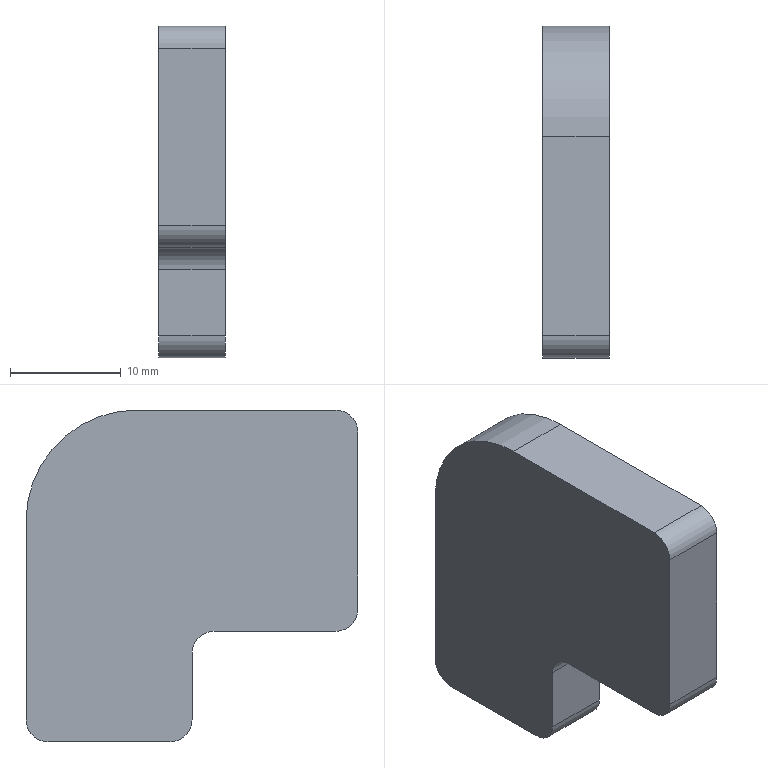Part | SolidWorks | features Fillet 1, FlatPattern 1, SMBaseFlange 1, SheetMetal 1 | 1 solid | 14 faces | box 6 x 30 x 30 mm | volume 4356 mm3 | plane 8 | cylinder 6 | commonest cylinder face diameters 4 x5 20 x1
STEP:
#1=CARTESIAN_POINT('',(0.,0.,-2.));
#2=VERTEX_POINT('',#1);
#3=CARTESIAN_POINT('',(0.,0.,-18.));
#4=VERTEX_POINT('',#3);
#5=CARTESIAN_POINT('',(0.,0.,-20.));
#6=DIRECTION('',(0.,0.,-1.));
#7=VECTOR('',#6,1000.);
#8=LINE('',#5,#7);
#9=EDGE_CURVE('',#2,#4,#8,.T.);
#10=ORIENTED_EDGE('',*,*,#9,.T.);
#11=CARTESIAN_POINT('',(6.,0.,-18.));
#12=VERTEX_POINT('',#11);
#13=CARTESIAN_POINT('',(6.,0.,-18.));
#14=DIRECTION('',(1.,0.,0.));
#15=VECTOR('',#14,1000.);
#16=LINE('',#13,#15);
#17=EDGE_CURVE('',#4,#12,#16,.T.);
#18=ORIENTED_EDGE('',*,*,#17,.T.);
#19=CARTESIAN_POINT('',(6.,0.,-2.));
#20=VERTEX_POINT('',#19);
#21=CARTESIAN_POINT('',(6.,0.,-20.));
#22=DIRECTION('',(0.,0.,-1.));
#23=VECTOR('',#22,1000.);
#24=LINE('',#21,#23);
#25=EDGE_CURVE('',#20,#12,#24,.T.);
#26=ORIENTED_EDGE('',*,*,#25,.F.);
#27=CARTESIAN_POINT('',(6.,0.,-2.));
#28=DIRECTION('',(-1.,0.,0.));
#29=VECTOR('',#28,1000.);
#30=LINE('',#27,#29);
#31=EDGE_CURVE('',#20,#2,#30,.T.);
#32=ORIENTED_EDGE('',*,*,#31,.T.);
#33=EDGE_LOOP('',(#10,#18,#26,#32));
#34=FACE_OUTER_BOUND('',#33,.T.);
#35=CARTESIAN_POINT('',(6.,0.,-20.));
#36=DIRECTION('',(0.,1.,0.));
#37=DIRECTION('',(0.,0.,1.));
#38=AXIS2_PLACEMENT_3D('',#35,#36,#37);
#39=PLANE('',#38);
#40=ADVANCED_FACE('',(#34),#39,.F.);
#41=CARTESIAN_POINT('',(0.,2.,-20.));
#42=VERTEX_POINT('',#41);
#43=CARTESIAN_POINT('',(0.,13.,-20.));
#44=VERTEX_POINT('',#43);
#45=CARTESIAN_POINT('',(0.,15.,-20.));
#46=DIRECTION('',(0.,1.,0.));
#47=VECTOR('',#46,1000.);
#48=LINE('',#45,#47);
#49=EDGE_CURVE('',#42,#44,#48,.T.);
#50=ORIENTED_EDGE('',*,*,#49,.T.);
#51=CARTESIAN_POINT('',(6.,13.,-20.));
#52=VERTEX_POINT('',#51);
#53=CARTESIAN_POINT('',(6.,13.,-20.));
#54=DIRECTION('',(1.,0.,0.));
#55=VECTOR('',#54,1000.);
#56=LINE('',#53,#55);
#57=EDGE_CURVE('',#44,#52,#56,.T.);
#58=ORIENTED_EDGE('',*,*,#57,.T.);
#59=CARTESIAN_POINT('',(6.,2.,-20.));
#60=VERTEX_POINT('',#59);
#61=CARTESIAN_POINT('',(6.,15.,-20.));
#62=DIRECTION('',(0.,1.,0.));
#63=VECTOR('',#62,1000.);
#64=LINE('',#61,#63);
#65=EDGE_CURVE('',#60,#52,#64,.T.);
#66=ORIENTED_EDGE('',*,*,#65,.F.);
#67=CARTESIAN_POINT('',(6.,2.,-20.));
#68=DIRECTION('',(-1.,0.,0.));
#69=VECTOR('',#68,1000.);
#70=LINE('',#67,#69);
#71=EDGE_CURVE('',#60,#42,#70,.T.);
#72=ORIENTED_EDGE('',*,*,#71,.T.);
#73=EDGE_LOOP('',(#50,#58,#66,#72));
#74=FACE_OUTER_BOUND('',#73,.T.);
#75=CARTESIAN_POINT('',(6.,15.,-20.));
#76=DIRECTION('',(0.,0.,1.));
#77=DIRECTION('',(1.,0.,0.));
#78=AXIS2_PLACEMENT_3D('',#75,#76,#77);
#79=PLANE('',#78);
#80=ADVANCED_FACE('',(#74),#79,.F.);
#81=CARTESIAN_POINT('',(6.,15.,-22.));
#82=VERTEX_POINT('',#81);
#83=CARTESIAN_POINT('',(6.,15.,-28.));
#84=VERTEX_POINT('',#83);
#85=CARTESIAN_POINT('',(6.,15.,-30.));
#86=DIRECTION('',(0.,0.,-1.));
#87=VECTOR('',#86,1000.);
#88=LINE('',#85,#87);
#89=EDGE_CURVE('',#82,#84,#88,.T.);
#90=ORIENTED_EDGE('',*,*,#89,.F.);
#91=CARTESIAN_POINT('',(0.,15.,-22.));
#92=VERTEX_POINT('',#91);
#93=CARTESIAN_POINT('',(0.,15.,-22.));
#94=DIRECTION('',(-1.,0.,0.));
#95=VECTOR('',#94,1000.);
#96=LINE('',#93,#95);
#97=EDGE_CURVE('',#82,#92,#96,.T.);
#98=ORIENTED_EDGE('',*,*,#97,.T.);
#99=CARTESIAN_POINT('',(0.,15.,-28.));
#100=VERTEX_POINT('',#99);
#101=CARTESIAN_POINT('',(0.,15.,-30.));
#102=DIRECTION('',(0.,0.,-1.));
#103=VECTOR('',#102,1000.);
#104=LINE('',#101,#103);
#105=EDGE_CURVE('',#92,#100,#104,.T.);
#106=ORIENTED_EDGE('',*,*,#105,.T.);
#107=CARTESIAN_POINT('',(6.,15.,-28.));
#108=DIRECTION('',(1.,0.,0.));
#109=VECTOR('',#108,1000.);
#110=LINE('',#107,#109);
#111=EDGE_CURVE('',#100,#84,#110,.T.);
#112=ORIENTED_EDGE('',*,*,#111,.T.);
#113=EDGE_LOOP('',(#90,#98,#106,#112));
#114=FACE_OUTER_BOUND('',#113,.T.);
#115=CARTESIAN_POINT('',(6.,15.,-30.));
#116=DIRECTION('',(0.,1.,0.));
#117=DIRECTION('',(0.,0.,1.));
#118=AXIS2_PLACEMENT_3D('',#115,#116,#117);
#119=PLANE('',#118);
#120=ADVANCED_FACE('',(#114),#119,.F.);
#121=CARTESIAN_POINT('',(0.,17.,-30.));
#122=VERTEX_POINT('',#121);
#123=CARTESIAN_POINT('',(0.,28.,-30.));
#124=VERTEX_POINT('',#123);
#125=CARTESIAN_POINT('',(0.,30.,-30.));
#126=DIRECTION('',(0.,1.,0.));
#127=VECTOR('',#126,1000.);
#128=LINE('',#125,#127);
#129=EDGE_CURVE('',#122,#124,#128,.T.);
#130=ORIENTED_EDGE('',*,*,#129,.T.);
#131=CARTESIAN_POINT('',(6.,28.,-30.));
#132=VERTEX_POINT('',#131);
#133=CARTESIAN_POINT('',(6.,28.,-30.));
#134=DIRECTION('',(1.,0.,0.));
#135=VECTOR('',#134,1000.);
#136=LINE('',#133,#135);
#137=EDGE_CURVE('',#124,#132,#136,.T.);
#138=ORIENTED_EDGE('',*,*,#137,.T.);
#139=CARTESIAN_POINT('',(6.,17.,-30.));
#140=VERTEX_POINT('',#139);
#141=CARTESIAN_POINT('',(6.,30.,-30.));
#142=DIRECTION('',(0.,1.,0.));
#143=VECTOR('',#142,1000.);
#144=LINE('',#141,#143);
#145=EDGE_CURVE('',#140,#132,#144,.T.);
#146=ORIENTED_EDGE('',*,*,#145,.F.);
#147=CARTESIAN_POINT('',(6.,17.,-30.));
#148=DIRECTION('',(-1.,0.,0.));
#149=VECTOR('',#148,1000.);
#150=LINE('',#147,#149);
#151=EDGE_CURVE('',#140,#122,#150,.T.);
#152=ORIENTED_EDGE('',*,*,#151,.T.);
#153=EDGE_LOOP('',(#130,#138,#146,#152));
#154=FACE_OUTER_BOUND('',#153,.T.);
#155=CARTESIAN_POINT('',(6.,30.,-30.));
#156=DIRECTION('',(0.,0.,1.));
#157=DIRECTION('',(0.,-1.,0.));
#158=AXIS2_PLACEMENT_3D('',#155,#156,#157);
#159=PLANE('',#158);
#160=ADVANCED_FACE('',(#154),#159,.F.);
#161=CARTESIAN_POINT('',(6.,30.,-28.));
#162=VERTEX_POINT('',#161);
#163=CARTESIAN_POINT('',(6.,30.,-10.));
#164=VERTEX_POINT('',#163);
#165=CARTESIAN_POINT('',(6.,30.,-10.));
#166=DIRECTION('',(0.,0.,1.));
#167=VECTOR('',#166,1000.);
#168=LINE('',#165,#167);
#169=EDGE_CURVE('',#162,#164,#168,.T.);
#170=ORIENTED_EDGE('',*,*,#169,.F.);
#171=CARTESIAN_POINT('',(0.,30.,-28.));
#172=VERTEX_POINT('',#171);
#173=CARTESIAN_POINT('',(6.,30.,-28.));
#174=DIRECTION('',(-1.,0.,0.));
#175=VECTOR('',#174,1000.);
#176=LINE('',#173,#175);
#177=EDGE_CURVE('',#162,#172,#176,.T.);
#178=ORIENTED_EDGE('',*,*,#177,.T.);
#179=CARTESIAN_POINT('',(0.,30.,-10.));
#180=VERTEX_POINT('',#179);
#181=CARTESIAN_POINT('',(0.,30.,-10.));
#182=DIRECTION('',(0.,0.,1.));
#183=VECTOR('',#182,1000.);
#184=LINE('',#181,#183);
#185=EDGE_CURVE('',#172,#180,#184,.T.);
#186=ORIENTED_EDGE('',*,*,#185,.T.);
#187=CARTESIAN_POINT('',(6.,30.,-10.));
#188=DIRECTION('',(-1.,0.,0.));
#189=VECTOR('',#188,1000.);
#190=LINE('',#187,#189);
#191=EDGE_CURVE('',#164,#180,#190,.T.);
#192=ORIENTED_EDGE('',*,*,#191,.F.);
#193=EDGE_LOOP('',(#170,#178,#186,#192));
#194=FACE_OUTER_BOUND('',#193,.T.);
#195=CARTESIAN_POINT('',(6.,30.,-10.));
#196=DIRECTION('',(0.,-1.,0.));
#197=DIRECTION('',(0.,0.,-1.));
#198=AXIS2_PLACEMENT_3D('',#195,#196,#197);
#199=PLANE('',#198);
#200=ADVANCED_FACE('',(#194),#199,.F.);
#201=CARTESIAN_POINT('',(0.,20.,0.));
#202=VERTEX_POINT('',#201);
#203=CARTESIAN_POINT('',(0.,20.,-10.));
#204=DIRECTION('',(1.,0.,0.));
#205=DIRECTION('',(0.,0.,1.));
#206=AXIS2_PLACEMENT_3D('',#203,#204,#205);
#207=CIRCLE('',#206,10.);
#208=EDGE_CURVE('',#180,#202,#207,.T.);
#209=ORIENTED_EDGE('',*,*,#208,.T.);
#210=CARTESIAN_POINT('',(6.,20.,0.));
#211=VERTEX_POINT('',#210);
#212=CARTESIAN_POINT('',(6.,20.,0.));
#213=DIRECTION('',(-1.,0.,0.));
#214=VECTOR('',#213,1000.);
#215=LINE('',#212,#214);
#216=EDGE_CURVE('',#211,#202,#215,.T.);
#217=ORIENTED_EDGE('',*,*,#216,.F.);
#218=CARTESIAN_POINT('',(6.,20.,-10.));
#219=DIRECTION('',(1.,0.,0.));
#220=DIRECTION('',(0.,0.,1.));
#221=AXIS2_PLACEMENT_3D('',#218,#219,#220);
#222=CIRCLE('',#221,10.);
#223=EDGE_CURVE('',#164,#211,#222,.T.);
#224=ORIENTED_EDGE('',*,*,#223,.F.);
#225=ORIENTED_EDGE('',*,*,#191,.T.);
#226=EDGE_LOOP('',(#209,#217,#224,#225));
#227=FACE_OUTER_BOUND('',#226,.T.);
#228=CARTESIAN_POINT('',(6.,20.,-10.));
#229=DIRECTION('',(-1.,0.,0.));
#230=DIRECTION('',(0.,0.,1.));
#231=AXIS2_PLACEMENT_3D('',#228,#229,#230);
#232=CYLINDRICAL_SURFACE('',#231,10.);
#233=ADVANCED_FACE('',(#227),#232,.T.);
#234=CARTESIAN_POINT('',(0.,2.,0.));
#235=VERTEX_POINT('',#234);
#236=CARTESIAN_POINT('',(0.,0.,0.));
#237=DIRECTION('',(0.,-1.,0.));
#238=VECTOR('',#237,1000.);
#239=LINE('',#236,#238);
#240=EDGE_CURVE('',#202,#235,#239,.T.);
#241=ORIENTED_EDGE('',*,*,#240,.T.);
#242=CARTESIAN_POINT('',(6.,2.,0.));
#243=VERTEX_POINT('',#242);
#244=CARTESIAN_POINT('',(6.,2.,0.));
#245=DIRECTION('',(1.,0.,0.));
#246=VECTOR('',#245,1000.);
#247=LINE('',#244,#246);
#248=EDGE_CURVE('',#235,#243,#247,.T.);
#249=ORIENTED_EDGE('',*,*,#248,.T.);
#250=CARTESIAN_POINT('',(6.,0.,0.));
#251=DIRECTION('',(0.,-1.,0.));
#252=VECTOR('',#251,1000.);
#253=LINE('',#250,#252);
#254=EDGE_CURVE('',#211,#243,#253,.T.);
#255=ORIENTED_EDGE('',*,*,#254,.F.);
#256=ORIENTED_EDGE('',*,*,#216,.T.);
#257=EDGE_LOOP('',(#241,#249,#255,#256));
#258=FACE_OUTER_BOUND('',#257,.T.);
#259=CARTESIAN_POINT('',(6.,0.,0.));
#260=DIRECTION('',(0.,0.,-1.));
#261=DIRECTION('',(-1.,0.,0.));
#262=AXIS2_PLACEMENT_3D('',#259,#260,#261);
#263=PLANE('',#262);
#264=ADVANCED_FACE('',(#258),#263,.F.);
#265=ORIENTED_EDGE('',*,*,#145,.T.);
#266=CARTESIAN_POINT('',(6.,28.,-28.));
#267=DIRECTION('',(1.,0.,0.));
#268=DIRECTION('',(0.,0.,1.));
#269=AXIS2_PLACEMENT_3D('',#266,#267,#268);
#270=CIRCLE('',#269,2.);
#271=EDGE_CURVE('',#132,#162,#270,.T.);
#272=ORIENTED_EDGE('',*,*,#271,.T.);
#273=ORIENTED_EDGE('',*,*,#169,.T.);
#274=ORIENTED_EDGE('',*,*,#223,.T.);
#275=ORIENTED_EDGE('',*,*,#254,.T.);
#276=CARTESIAN_POINT('',(6.,2.,-2.));
#277=DIRECTION('',(1.,0.,0.));
#278=DIRECTION('',(0.,0.,1.));
#279=AXIS2_PLACEMENT_3D('',#276,#277,#278);
#280=CIRCLE('',#279,2.);
#281=EDGE_CURVE('',#243,#20,#280,.T.);
#282=ORIENTED_EDGE('',*,*,#281,.T.);
#283=ORIENTED_EDGE('',*,*,#25,.T.);
#284=CARTESIAN_POINT('',(6.,2.,-18.));
#285=DIRECTION('',(1.,0.,0.));
#286=DIRECTION('',(0.,0.,1.));
#287=AXIS2_PLACEMENT_3D('',#284,#285,#286);
#288=CIRCLE('',#287,2.);
#289=EDGE_CURVE('',#12,#60,#288,.T.);
#290=ORIENTED_EDGE('',*,*,#289,.T.);
#291=ORIENTED_EDGE('',*,*,#65,.T.);
#292=CARTESIAN_POINT('',(6.,13.,-22.));
#293=DIRECTION('',(-1.,0.,0.));
#294=DIRECTION('',(0.,0.,1.));
#295=AXIS2_PLACEMENT_3D('',#292,#293,#294);
#296=CIRCLE('',#295,2.);
#297=EDGE_CURVE('',#52,#82,#296,.T.);
#298=ORIENTED_EDGE('',*,*,#297,.T.);
#299=ORIENTED_EDGE('',*,*,#89,.T.);
#300=CARTESIAN_POINT('',(6.,17.,-28.));
#301=DIRECTION('',(1.,0.,0.));
#302=DIRECTION('',(0.,0.,1.));
#303=AXIS2_PLACEMENT_3D('',#300,#301,#302);
#304=CIRCLE('',#303,2.);
#305=EDGE_CURVE('',#84,#140,#304,.T.);
#306=ORIENTED_EDGE('',*,*,#305,.T.);
#307=EDGE_LOOP('',(#265,#272,#273,#274,#275,#282,#283,#290,#291,#298,#299,#306));
#308=FACE_OUTER_BOUND('',#307,.T.);
#309=CARTESIAN_POINT('',(6.,20.,-10.));
#310=DIRECTION('',(-1.,0.,0.));
#311=DIRECTION('',(0.,0.,1.));
#312=AXIS2_PLACEMENT_3D('',#309,#310,#311);
#313=PLANE('',#312);
#314=ADVANCED_FACE('',(#308),#313,.F.);
#315=ORIENTED_EDGE('',*,*,#185,.F.);
#316=CARTESIAN_POINT('',(0.,28.,-28.));
#317=DIRECTION('',(-1.,0.,0.));
#318=DIRECTION('',(0.,0.,1.));
#319=AXIS2_PLACEMENT_3D('',#316,#317,#318);
#320=CIRCLE('',#319,2.);
#321=EDGE_CURVE('',#172,#124,#320,.T.);
#322=ORIENTED_EDGE('',*,*,#321,.T.);
#323=ORIENTED_EDGE('',*,*,#129,.F.);
#324=CARTESIAN_POINT('',(0.,17.,-28.));
#325=DIRECTION('',(-1.,0.,0.));
#326=DIRECTION('',(0.,0.,1.));
#327=AXIS2_PLACEMENT_3D('',#324,#325,#326);
#328=CIRCLE('',#327,2.);
#329=EDGE_CURVE('',#122,#100,#328,.T.);
#330=ORIENTED_EDGE('',*,*,#329,.T.);
#331=ORIENTED_EDGE('',*,*,#105,.F.);
#332=CARTESIAN_POINT('',(0.,13.,-22.));
#333=DIRECTION('',(1.,0.,0.));
#334=DIRECTION('',(0.,0.,1.));
#335=AXIS2_PLACEMENT_3D('',#332,#333,#334);
#336=CIRCLE('',#335,2.);
#337=EDGE_CURVE('',#92,#44,#336,.T.);
#338=ORIENTED_EDGE('',*,*,#337,.T.);
#339=ORIENTED_EDGE('',*,*,#49,.F.);
#340=CARTESIAN_POINT('',(0.,2.,-18.));
#341=DIRECTION('',(-1.,0.,0.));
#342=DIRECTION('',(0.,0.,1.));
#343=AXIS2_PLACEMENT_3D('',#340,#341,#342);
#344=CIRCLE('',#343,2.);
#345=EDGE_CURVE('',#42,#4,#344,.T.);
#346=ORIENTED_EDGE('',*,*,#345,.T.);
#347=ORIENTED_EDGE('',*,*,#9,.F.);
#348=CARTESIAN_POINT('',(0.,2.,-2.));
#349=DIRECTION('',(-1.,0.,0.));
#350=DIRECTION('',(0.,0.,1.));
#351=AXIS2_PLACEMENT_3D('',#348,#349,#350);
#352=CIRCLE('',#351,2.);
#353=EDGE_CURVE('',#2,#235,#352,.T.);
#354=ORIENTED_EDGE('',*,*,#353,.T.);
#355=ORIENTED_EDGE('',*,*,#240,.F.);
#356=ORIENTED_EDGE('',*,*,#208,.F.);
#357=EDGE_LOOP('',(#315,#322,#323,#330,#331,#338,#339,#346,#347,#354,#355,#356));
#358=FACE_OUTER_BOUND('',#357,.T.);
#359=CARTESIAN_POINT('',(0.,20.,-10.));
#360=DIRECTION('',(-1.,0.,0.));
#361=DIRECTION('',(0.,0.,1.));
#362=AXIS2_PLACEMENT_3D('',#359,#360,#361);
#363=PLANE('',#362);
#364=ADVANCED_FACE('',(#358),#363,.T.);
#365=ORIENTED_EDGE('',*,*,#297,.F.);
#366=ORIENTED_EDGE('',*,*,#57,.F.);
#367=ORIENTED_EDGE('',*,*,#337,.F.);
#368=ORIENTED_EDGE('',*,*,#97,.F.);
#369=EDGE_LOOP('',(#365,#366,#367,#368));
#370=FACE_OUTER_BOUND('',#369,.T.);
#371=CARTESIAN_POINT('',(6.,13.,-22.));
#372=DIRECTION('',(1.,0.,0.));
#373=DIRECTION('',(0.,0.,-1.));
#374=AXIS2_PLACEMENT_3D('',#371,#372,#373);
#375=CYLINDRICAL_SURFACE('',#374,2.);
#376=ADVANCED_FACE('',(#370),#375,.F.);
#377=ORIENTED_EDGE('',*,*,#271,.F.);
#378=ORIENTED_EDGE('',*,*,#137,.F.);
#379=ORIENTED_EDGE('',*,*,#321,.F.);
#380=ORIENTED_EDGE('',*,*,#177,.F.);
#381=EDGE_LOOP('',(#377,#378,#379,#380));
#382=FACE_OUTER_BOUND('',#381,.T.);
#383=CARTESIAN_POINT('',(6.,28.,-28.));
#384=DIRECTION('',(-1.,0.,0.));
#385=DIRECTION('',(0.,0.,1.));
#386=AXIS2_PLACEMENT_3D('',#383,#384,#385);
#387=CYLINDRICAL_SURFACE('',#386,2.);
#388=ADVANCED_FACE('',(#382),#387,.T.);
#389=ORIENTED_EDGE('',*,*,#305,.F.);
#390=ORIENTED_EDGE('',*,*,#111,.F.);
#391=ORIENTED_EDGE('',*,*,#329,.F.);
#392=ORIENTED_EDGE('',*,*,#151,.F.);
#393=EDGE_LOOP('',(#389,#390,#391,#392));
#394=FACE_OUTER_BOUND('',#393,.T.);
#395=CARTESIAN_POINT('',(6.,17.,-28.));
#396=DIRECTION('',(-1.,0.,0.));
#397=DIRECTION('',(0.,0.,1.));
#398=AXIS2_PLACEMENT_3D('',#395,#396,#397);
#399=CYLINDRICAL_SURFACE('',#398,2.);
#400=ADVANCED_FACE('',(#394),#399,.T.);
#401=ORIENTED_EDGE('',*,*,#289,.F.);
#402=ORIENTED_EDGE('',*,*,#17,.F.);
#403=ORIENTED_EDGE('',*,*,#345,.F.);
#404=ORIENTED_EDGE('',*,*,#71,.F.);
#405=EDGE_LOOP('',(#401,#402,#403,#404));
#406=FACE_OUTER_BOUND('',#405,.T.);
#407=CARTESIAN_POINT('',(6.,2.,-18.));
#408=DIRECTION('',(-1.,0.,0.));
#409=DIRECTION('',(0.,0.,1.));
#410=AXIS2_PLACEMENT_3D('',#407,#408,#409);
#411=CYLINDRICAL_SURFACE('',#410,2.);
#412=ADVANCED_FACE('',(#406),#411,.T.);
#413=ORIENTED_EDGE('',*,*,#281,.F.);
#414=ORIENTED_EDGE('',*,*,#248,.F.);
#415=ORIENTED_EDGE('',*,*,#353,.F.);
#416=ORIENTED_EDGE('',*,*,#31,.F.);
#417=EDGE_LOOP('',(#413,#414,#415,#416));
#418=FACE_OUTER_BOUND('',#417,.T.);
#419=CARTESIAN_POINT('',(6.,2.,-2.));
#420=DIRECTION('',(-1.,0.,0.));
#421=DIRECTION('',(0.,0.,1.));
#422=AXIS2_PLACEMENT_3D('',#419,#420,#421);
#423=CYLINDRICAL_SURFACE('',#422,2.);
#424=ADVANCED_FACE('',(#418),#423,.T.);
#425=CLOSED_SHELL('',(#40,#80,#120,#160,#200,#233,#264,#314,#364,#376,#388,#400,#412,#424));
#426=MANIFOLD_SOLID_BREP('',#425);
#427=CARTESIAN_POINT('',(0.,0.,0.));
#428=DIRECTION('',(0.,0.,1.));
#429=DIRECTION('',(1.,0.,0.));
#430=AXIS2_PLACEMENT_3D('',#427,#428,#429);
#431=(LENGTH_UNIT()NAMED_UNIT(*)SI_UNIT(.MILLI.,.METRE.));
#432=UNCERTAINTY_MEASURE_WITH_UNIT(LENGTH_MEASURE(0.00001),#431,'','');
#433=(NAMED_UNIT(*)PLANE_ANGLE_UNIT()SI_UNIT($,.RADIAN.));
#434=(NAMED_UNIT(*)SI_UNIT($,.STERADIAN.)SOLID_ANGLE_UNIT());
#435=(GEOMETRIC_REPRESENTATION_CONTEXT(3)GLOBAL_UNCERTAINTY_ASSIGNED_CONTEXT((#432))GLOBAL_UNIT_ASSIGNED_CONTEXT((#431,#433,#434))REPRESENTATION_CONTEXT('',''));
#436=ADVANCED_BREP_SHAPE_REPRESENTATION('',(#426,#430),#435);